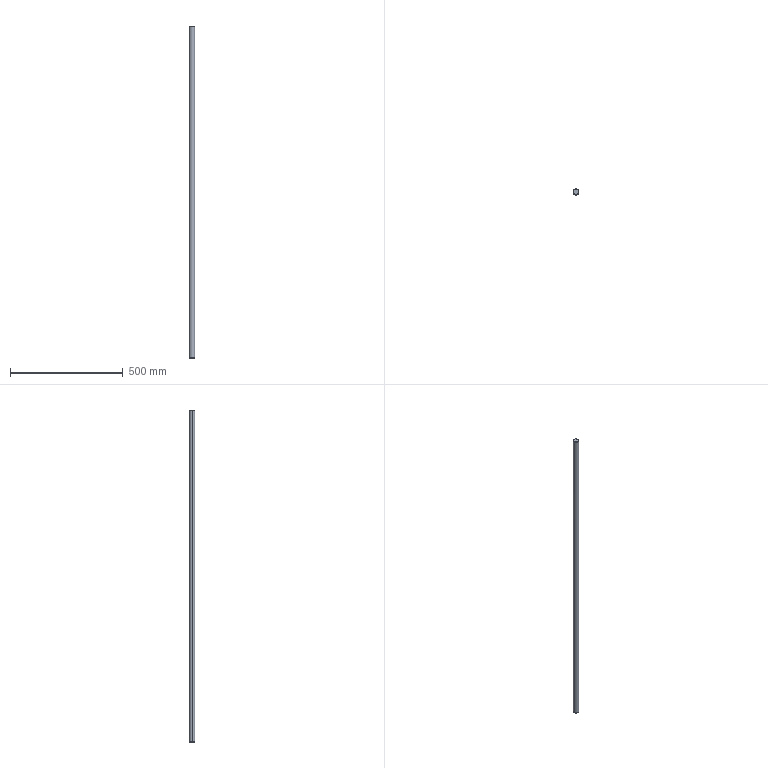Part | STEP file | 1 solid | 8 faces | box 25 x 25 x 1470 mm | volume 721508 mm3 | cone 4 | cylinder 2 | plane 2 | commonest cylinder face diameters 25 x2
STEP:
#1=CARTESIAN_POINT('',(0.,0.,0.));
#2=DIRECTION('',(0.,0.,1.));
#3=DIRECTION('',(1.,0.,0.));
#4=AXIS2_PLACEMENT_3D('',#1,#2,#3);
#5=CARTESIAN_POINT('',(-11.5,0.,-755.));
#6=VERTEX_POINT('',#5);
#7=CARTESIAN_POINT('',(11.5,0.,-755.));
#8=VERTEX_POINT('',#7);
#9=CARTESIAN_POINT('',(0.,0.,-755.));
#10=DIRECTION('',(0.,0.,-1.));
#11=DIRECTION('',(1.,0.,0.));
#12=AXIS2_PLACEMENT_3D('',#9,#10,#11);
#13=CIRCLE('',#12,11.5);
#14=CARTESIAN_POINT('',(0.,0.,-754.));
#15=DIRECTION('',(0.,0.,1.));
#16=DIRECTION('',(1.,0.,0.));
#17=AXIS2_PLACEMENT_3D('',#14,#15,#16);
#18=CONICAL_SURFACE('',#17,12.5,0.7854);
#19=CARTESIAN_POINT('',(6.283,-1.));
#20=DIRECTION('',(-1.,0.));
#21=VECTOR('',#20,1.);
#22=LINE('',#19,#21);
#23=(GEOMETRIC_REPRESENTATION_CONTEXT(2)PARAMETRIC_REPRESENTATION_CONTEXT()REPRESENTATION_CONTEXT('',''));
#24=DEFINITIONAL_REPRESENTATION('',(#22),#23);
#25=PCURVE('',#18,#24);
#26=CARTESIAN_POINT('',(0.,0.,-755.));
#27=DIRECTION('',(0.,0.,1.));
#28=DIRECTION('',(1.,0.,0.));
#29=AXIS2_PLACEMENT_3D('',#26,#27,#28);
#30=PLANE('',#29);
#31=CARTESIAN_POINT('',(11.5,0.));
#32=CARTESIAN_POINT('',(11.5,-19.919));
#33=CARTESIAN_POINT('',(-5.75,-9.959));
#34=CARTESIAN_POINT('',(-23.,0.));
#35=CARTESIAN_POINT('',(-5.75,9.959));
#36=CARTESIAN_POINT('',(11.5,19.919));
#37=CARTESIAN_POINT('',(11.5,0.));
#38=(BOUNDED_CURVE()B_SPLINE_CURVE(2,(#31,#32,#33,#34,#35,#36,#37),.UNSPECIFIED.,.T.,.F.)B_SPLINE_CURVE_WITH_KNOTS((1,2,2,2,2,1),(-2.094,0.,2.094,4.189,6.283,8.378),.UNSPECIFIED.)CURVE()GEOMETRIC_REPRESENTATION_ITEM()RATIONAL_B_SPLINE_CURVE((1.,0.5,1.,0.5,1.,0.5,1.))REPRESENTATION_ITEM(''));
#39=(GEOMETRIC_REPRESENTATION_CONTEXT(2)PARAMETRIC_REPRESENTATION_CONTEXT()REPRESENTATION_CONTEXT('',''));
#40=DEFINITIONAL_REPRESENTATION('',(#38),#39);
#41=PCURVE('',#30,#40);
#42=SURFACE_CURVE('',#13,(#25,#41),.PCURVE_S1.);
#43=EDGE_CURVE('',#6,#8,#42,.T.);
#44=ORIENTED_EDGE('',*,*,#43,.F.);
#45=CARTESIAN_POINT('',(-12.5,0.,-754.));
#46=VERTEX_POINT('',#45);
#47=CARTESIAN_POINT('',(-12.5,0.,-754.));
#48=DIRECTION('',(-0.7071,0.,0.7071));
#49=VECTOR('',#48,1.);
#50=LINE('',#47,#49);
#51=CARTESIAN_POINT('',(3.142,0.));
#52=DIRECTION('',(0.,1.));
#53=VECTOR('',#52,1.);
#54=LINE('',#51,#53);
#55=(GEOMETRIC_REPRESENTATION_CONTEXT(2)PARAMETRIC_REPRESENTATION_CONTEXT()REPRESENTATION_CONTEXT('',''));
#56=DEFINITIONAL_REPRESENTATION('',(#54),#55);
#57=PCURVE('',#18,#56);
#58=CARTESIAN_POINT('',(0.,0.,-754.));
#59=DIRECTION('',(0.,0.,1.));
#60=DIRECTION('',(1.,0.,0.));
#61=AXIS2_PLACEMENT_3D('',#58,#59,#60);
#62=CONICAL_SURFACE('',#61,12.5,0.7854);
#63=CARTESIAN_POINT('',(3.142,0.));
#64=DIRECTION('',(0.,1.));
#65=VECTOR('',#64,1.);
#66=LINE('',#63,#65);
#67=(GEOMETRIC_REPRESENTATION_CONTEXT(2)PARAMETRIC_REPRESENTATION_CONTEXT()REPRESENTATION_CONTEXT('',''));
#68=DEFINITIONAL_REPRESENTATION('',(#66),#67);
#69=PCURVE('',#62,#68);
#70=SURFACE_CURVE('',#50,(#57,#69),.PCURVE_S1.);
#71=EDGE_CURVE('',#6,#46,#70,.T.);
#72=ORIENTED_EDGE('',*,*,#71,.T.);
#73=CARTESIAN_POINT('',(12.5,0.,-754.));
#74=VERTEX_POINT('',#73);
#75=CARTESIAN_POINT('',(0.,0.,-754.));
#76=DIRECTION('',(0.,0.,1.));
#77=DIRECTION('',(1.,0.,0.));
#78=AXIS2_PLACEMENT_3D('',#75,#76,#77);
#79=CIRCLE('',#78,12.5);
#80=CARTESIAN_POINT('',(0.,0.));
#81=DIRECTION('',(1.,0.));
#82=VECTOR('',#81,1.);
#83=LINE('',#80,#82);
#84=(GEOMETRIC_REPRESENTATION_CONTEXT(2)PARAMETRIC_REPRESENTATION_CONTEXT()REPRESENTATION_CONTEXT('',''));
#85=DEFINITIONAL_REPRESENTATION('',(#83),#84);
#86=PCURVE('',#18,#85);
#87=CARTESIAN_POINT('',(0.,0.,755.));
#88=DIRECTION('',(0.,0.,-1.));
#89=DIRECTION('',(-1.,0.,0.));
#90=AXIS2_PLACEMENT_3D('',#87,#88,#89);
#91=CYLINDRICAL_SURFACE('',#90,12.5);
#92=CARTESIAN_POINT('',(3.142,1509.));
#93=DIRECTION('',(-1.,0.));
#94=VECTOR('',#93,1.);
#95=LINE('',#92,#94);
#96=(GEOMETRIC_REPRESENTATION_CONTEXT(2)PARAMETRIC_REPRESENTATION_CONTEXT()REPRESENTATION_CONTEXT('',''));
#97=DEFINITIONAL_REPRESENTATION('',(#95),#96);
#98=PCURVE('',#91,#97);
#99=SURFACE_CURVE('',#79,(#86,#98),.PCURVE_S1.);
#100=EDGE_CURVE('',#74,#46,#99,.T.);
#101=ORIENTED_EDGE('',*,*,#100,.F.);
#102=CARTESIAN_POINT('',(12.5,0.,-754.));
#103=DIRECTION('',(0.7071,0.,0.7071));
#104=VECTOR('',#103,1.);
#105=LINE('',#102,#104);
#106=CARTESIAN_POINT('',(0.,0.));
#107=DIRECTION('',(0.,1.));
#108=VECTOR('',#107,1.);
#109=LINE('',#106,#108);
#110=(GEOMETRIC_REPRESENTATION_CONTEXT(2)PARAMETRIC_REPRESENTATION_CONTEXT()REPRESENTATION_CONTEXT('',''));
#111=DEFINITIONAL_REPRESENTATION('',(#109),#110);
#112=PCURVE('',#18,#111);
#113=CARTESIAN_POINT('',(6.283,0.));
#114=DIRECTION('',(0.,1.));
#115=VECTOR('',#114,1.);
#116=LINE('',#113,#115);
#117=(GEOMETRIC_REPRESENTATION_CONTEXT(2)PARAMETRIC_REPRESENTATION_CONTEXT()REPRESENTATION_CONTEXT('',''));
#118=DEFINITIONAL_REPRESENTATION('',(#116),#117);
#119=PCURVE('',#62,#118);
#120=SURFACE_CURVE('',#105,(#112,#119),.PCURVE_S1.);
#121=EDGE_CURVE('',#8,#74,#120,.T.);
#122=ORIENTED_EDGE('',*,*,#121,.F.);
#123=EDGE_LOOP('',(#44,#72,#101,#122));
#124=FACE_BOUND('',#123,.T.);
#125=ADVANCED_FACE('',(#124),#18,.T.);
#126=CARTESIAN_POINT('',(11.5,0.,715.));
#127=VERTEX_POINT('',#126);
#128=CARTESIAN_POINT('',(-11.5,0.,715.));
#129=VERTEX_POINT('',#128);
#130=CARTESIAN_POINT('',(0.,0.,715.));
#131=DIRECTION('',(0.,0.,1.));
#132=DIRECTION('',(1.,0.,0.));
#133=AXIS2_PLACEMENT_3D('',#130,#131,#132);
#134=CIRCLE('',#133,11.5);
#135=CARTESIAN_POINT('',(0.,0.,715.));
#136=DIRECTION('',(0.,0.,-1.));
#137=DIRECTION('',(-1.,0.,0.));
#138=AXIS2_PLACEMENT_3D('',#135,#136,#137);
#139=CONICAL_SURFACE('',#138,11.5,0.7854);
#140=CARTESIAN_POINT('',(3.142,0.));
#141=DIRECTION('',(-1.,0.));
#142=VECTOR('',#141,1.);
#143=LINE('',#140,#142);
#144=(GEOMETRIC_REPRESENTATION_CONTEXT(2)PARAMETRIC_REPRESENTATION_CONTEXT()REPRESENTATION_CONTEXT('',''));
#145=DEFINITIONAL_REPRESENTATION('',(#143),#144);
#146=PCURVE('',#139,#145);
#147=CARTESIAN_POINT('',(0.,0.,715.));
#148=DIRECTION('',(0.,0.,1.));
#149=DIRECTION('',(1.,0.,0.));
#150=AXIS2_PLACEMENT_3D('',#147,#148,#149);
#151=PLANE('',#150);
#152=CARTESIAN_POINT('',(0.,0.));
#153=DIRECTION('',(1.,0.));
#154=AXIS2_PLACEMENT_2D('',#152,#153);
#155=CIRCLE('',#154,11.5);
#156=(GEOMETRIC_REPRESENTATION_CONTEXT(2)PARAMETRIC_REPRESENTATION_CONTEXT()REPRESENTATION_CONTEXT('',''));
#157=DEFINITIONAL_REPRESENTATION('',(#155),#156);
#158=PCURVE('',#151,#157);
#159=SURFACE_CURVE('',#134,(#146,#158),.PCURVE_S1.);
#160=EDGE_CURVE('',#127,#129,#159,.T.);
#161=ORIENTED_EDGE('',*,*,#160,.F.);
#162=CARTESIAN_POINT('',(12.5,0.,714.));
#163=VERTEX_POINT('',#162);
#164=CARTESIAN_POINT('',(11.5,0.,715.));
#165=DIRECTION('',(0.7071,0.,-0.7071));
#166=VECTOR('',#165,1.);
#167=LINE('',#164,#166);
#168=CARTESIAN_POINT('',(3.142,0.));
#169=DIRECTION('',(0.,1.));
#170=VECTOR('',#169,1.);
#171=LINE('',#168,#170);
#172=(GEOMETRIC_REPRESENTATION_CONTEXT(2)PARAMETRIC_REPRESENTATION_CONTEXT()REPRESENTATION_CONTEXT('',''));
#173=DEFINITIONAL_REPRESENTATION('',(#171),#172);
#174=PCURVE('',#139,#173);
#175=CARTESIAN_POINT('',(0.,0.,715.));
#176=DIRECTION('',(0.,0.,-1.));
#177=DIRECTION('',(-1.,0.,0.));
#178=AXIS2_PLACEMENT_3D('',#175,#176,#177);
#179=CONICAL_SURFACE('',#178,11.5,0.7854);
#180=CARTESIAN_POINT('',(3.142,0.));
#181=DIRECTION('',(0.,1.));
#182=VECTOR('',#181,1.);
#183=LINE('',#180,#182);
#184=(GEOMETRIC_REPRESENTATION_CONTEXT(2)PARAMETRIC_REPRESENTATION_CONTEXT()REPRESENTATION_CONTEXT('',''));
#185=DEFINITIONAL_REPRESENTATION('',(#183),#184);
#186=PCURVE('',#179,#185);
#187=SURFACE_CURVE('',#167,(#174,#186),.PCURVE_S1.);
#188=EDGE_CURVE('',#127,#163,#187,.T.);
#189=ORIENTED_EDGE('',*,*,#188,.T.);
#190=CARTESIAN_POINT('',(-12.5,0.,714.));
#191=VERTEX_POINT('',#190);
#192=CARTESIAN_POINT('',(0.,0.,714.));
#193=DIRECTION('',(0.,0.,-1.));
#194=DIRECTION('',(1.,0.,0.));
#195=AXIS2_PLACEMENT_3D('',#192,#193,#194);
#196=CIRCLE('',#195,12.5);
#197=CARTESIAN_POINT('',(-3.142,1.));
#198=DIRECTION('',(1.,0.));
#199=VECTOR('',#198,1.);
#200=LINE('',#197,#199);
#201=(GEOMETRIC_REPRESENTATION_CONTEXT(2)PARAMETRIC_REPRESENTATION_CONTEXT()REPRESENTATION_CONTEXT('',''));
#202=DEFINITIONAL_REPRESENTATION('',(#200),#201);
#203=PCURVE('',#139,#202);
#204=CARTESIAN_POINT('',(-3.142,41.));
#205=DIRECTION('',(1.,0.));
#206=VECTOR('',#205,1.);
#207=LINE('',#204,#206);
#208=(GEOMETRIC_REPRESENTATION_CONTEXT(2)PARAMETRIC_REPRESENTATION_CONTEXT()REPRESENTATION_CONTEXT('',''));
#209=DEFINITIONAL_REPRESENTATION('',(#207),#208);
#210=PCURVE('',#91,#209);
#211=SURFACE_CURVE('',#196,(#203,#210),.PCURVE_S1.);
#212=EDGE_CURVE('',#191,#163,#211,.T.);
#213=ORIENTED_EDGE('',*,*,#212,.F.);
#214=CARTESIAN_POINT('',(-11.5,0.,715.));
#215=DIRECTION('',(-0.7071,0.,-0.7071));
#216=VECTOR('',#215,1.);
#217=LINE('',#214,#216);
#218=CARTESIAN_POINT('',(0.,0.));
#219=DIRECTION('',(0.,1.));
#220=VECTOR('',#219,1.);
#221=LINE('',#218,#220);
#222=(GEOMETRIC_REPRESENTATION_CONTEXT(2)PARAMETRIC_REPRESENTATION_CONTEXT()REPRESENTATION_CONTEXT('',''));
#223=DEFINITIONAL_REPRESENTATION('',(#221),#222);
#224=PCURVE('',#139,#223);
#225=CARTESIAN_POINT('',(6.283,0.));
#226=DIRECTION('',(0.,1.));
#227=VECTOR('',#226,1.);
#228=LINE('',#225,#227);
#229=(GEOMETRIC_REPRESENTATION_CONTEXT(2)PARAMETRIC_REPRESENTATION_CONTEXT()REPRESENTATION_CONTEXT('',''));
#230=DEFINITIONAL_REPRESENTATION('',(#228),#229);
#231=PCURVE('',#179,#230);
#232=SURFACE_CURVE('',#217,(#224,#231),.PCURVE_S1.);
#233=EDGE_CURVE('',#129,#191,#232,.T.);
#234=ORIENTED_EDGE('',*,*,#233,.F.);
#235=EDGE_LOOP('',(#161,#189,#213,#234));
#236=FACE_BOUND('',#235,.T.);
#237=ADVANCED_FACE('',(#236),#139,.T.);
#238=ORIENTED_EDGE('',*,*,#212,.T.);
#239=CARTESIAN_POINT('',(12.5,0.,755.));
#240=DIRECTION('',(0.,0.,-1.));
#241=VECTOR('',#240,1.);
#242=LINE('',#239,#241);
#243=CARTESIAN_POINT('',(3.142,0.));
#244=DIRECTION('',(0.,1.));
#245=VECTOR('',#244,1.);
#246=LINE('',#243,#245);
#247=(GEOMETRIC_REPRESENTATION_CONTEXT(2)PARAMETRIC_REPRESENTATION_CONTEXT()REPRESENTATION_CONTEXT('',''));
#248=DEFINITIONAL_REPRESENTATION('',(#246),#247);
#249=PCURVE('',#91,#248);
#250=CARTESIAN_POINT('',(0.,0.,755.));
#251=DIRECTION('',(0.,0.,-1.));
#252=DIRECTION('',(-1.,0.,0.));
#253=AXIS2_PLACEMENT_3D('',#250,#251,#252);
#254=CYLINDRICAL_SURFACE('',#253,12.5);
#255=CARTESIAN_POINT('',(3.142,0.));
#256=DIRECTION('',(0.,1.));
#257=VECTOR('',#256,1.);
#258=LINE('',#255,#257);
#259=(GEOMETRIC_REPRESENTATION_CONTEXT(2)PARAMETRIC_REPRESENTATION_CONTEXT()REPRESENTATION_CONTEXT('',''));
#260=DEFINITIONAL_REPRESENTATION('',(#258),#259);
#261=PCURVE('',#254,#260);
#262=SURFACE_CURVE('',#242,(#249,#261),.PCURVE_S1.);
#263=EDGE_CURVE('',#163,#74,#262,.T.);
#264=ORIENTED_EDGE('',*,*,#263,.T.);
#265=ORIENTED_EDGE('',*,*,#100,.T.);
#266=CARTESIAN_POINT('',(-12.5,0.,755.));
#267=DIRECTION('',(0.,0.,-1.));
#268=VECTOR('',#267,1.);
#269=LINE('',#266,#268);
#270=CARTESIAN_POINT('',(0.,0.));
#271=DIRECTION('',(0.,1.));
#272=VECTOR('',#271,1.);
#273=LINE('',#270,#272);
#274=(GEOMETRIC_REPRESENTATION_CONTEXT(2)PARAMETRIC_REPRESENTATION_CONTEXT()REPRESENTATION_CONTEXT('',''));
#275=DEFINITIONAL_REPRESENTATION('',(#273),#274);
#276=PCURVE('',#91,#275);
#277=CARTESIAN_POINT('',(6.283,0.));
#278=DIRECTION('',(0.,1.));
#279=VECTOR('',#278,1.);
#280=LINE('',#277,#279);
#281=(GEOMETRIC_REPRESENTATION_CONTEXT(2)PARAMETRIC_REPRESENTATION_CONTEXT()REPRESENTATION_CONTEXT('',''));
#282=DEFINITIONAL_REPRESENTATION('',(#280),#281);
#283=PCURVE('',#254,#282);
#284=SURFACE_CURVE('',#269,(#276,#283),.PCURVE_S1.);
#285=EDGE_CURVE('',#191,#46,#284,.T.);
#286=ORIENTED_EDGE('',*,*,#285,.F.);
#287=EDGE_LOOP('',(#238,#264,#265,#286));
#288=FACE_BOUND('',#287,.T.);
#289=ADVANCED_FACE('',(#288),#91,.T.);
#290=ORIENTED_EDGE('',*,*,#263,.F.);
#291=CARTESIAN_POINT('',(0.,0.,714.));
#292=DIRECTION('',(0.,0.,-1.));
#293=DIRECTION('',(1.,0.,0.));
#294=AXIS2_PLACEMENT_3D('',#291,#292,#293);
#295=CIRCLE('',#294,12.5);
#296=CARTESIAN_POINT('',(3.142,41.));
#297=DIRECTION('',(1.,0.));
#298=VECTOR('',#297,1.);
#299=LINE('',#296,#298);
#300=(GEOMETRIC_REPRESENTATION_CONTEXT(2)PARAMETRIC_REPRESENTATION_CONTEXT()REPRESENTATION_CONTEXT('',''));
#301=DEFINITIONAL_REPRESENTATION('',(#299),#300);
#302=PCURVE('',#254,#301);
#303=CARTESIAN_POINT('',(3.142,1.));
#304=DIRECTION('',(1.,0.));
#305=VECTOR('',#304,1.);
#306=LINE('',#303,#305);
#307=(GEOMETRIC_REPRESENTATION_CONTEXT(2)PARAMETRIC_REPRESENTATION_CONTEXT()REPRESENTATION_CONTEXT('',''));
#308=DEFINITIONAL_REPRESENTATION('',(#306),#307);
#309=PCURVE('',#179,#308);
#310=SURFACE_CURVE('',#295,(#302,#309),.PCURVE_S1.);
#311=EDGE_CURVE('',#163,#191,#310,.T.);
#312=ORIENTED_EDGE('',*,*,#311,.T.);
#313=ORIENTED_EDGE('',*,*,#285,.T.);
#314=CARTESIAN_POINT('',(0.,0.,-754.));
#315=DIRECTION('',(0.,0.,1.));
#316=DIRECTION('',(1.,0.,0.));
#317=AXIS2_PLACEMENT_3D('',#314,#315,#316);
#318=CIRCLE('',#317,12.5);
#319=CARTESIAN_POINT('',(9.425,1509.));
#320=DIRECTION('',(-1.,0.));
#321=VECTOR('',#320,1.);
#322=LINE('',#319,#321);
#323=(GEOMETRIC_REPRESENTATION_CONTEXT(2)PARAMETRIC_REPRESENTATION_CONTEXT()REPRESENTATION_CONTEXT('',''));
#324=DEFINITIONAL_REPRESENTATION('',(#322),#323);
#325=PCURVE('',#254,#324);
#326=CARTESIAN_POINT('',(0.,0.));
#327=DIRECTION('',(1.,0.));
#328=VECTOR('',#327,1.);
#329=LINE('',#326,#328);
#330=(GEOMETRIC_REPRESENTATION_CONTEXT(2)PARAMETRIC_REPRESENTATION_CONTEXT()REPRESENTATION_CONTEXT('',''));
#331=DEFINITIONAL_REPRESENTATION('',(#329),#330);
#332=PCURVE('',#62,#331);
#333=SURFACE_CURVE('',#318,(#325,#332),.PCURVE_S1.);
#334=EDGE_CURVE('',#46,#74,#333,.T.);
#335=ORIENTED_EDGE('',*,*,#334,.T.);
#336=EDGE_LOOP('',(#290,#312,#313,#335));
#337=FACE_BOUND('',#336,.T.);
#338=ADVANCED_FACE('',(#337),#254,.T.);
#339=CARTESIAN_POINT('',(0.,0.,715.));
#340=DIRECTION('',(0.,0.,1.));
#341=DIRECTION('',(1.,0.,0.));
#342=AXIS2_PLACEMENT_3D('',#339,#340,#341);
#343=CIRCLE('',#342,11.5);
#344=CARTESIAN_POINT('',(0.,0.));
#345=DIRECTION('',(1.,0.));
#346=AXIS2_PLACEMENT_2D('',#344,#345);
#347=CIRCLE('',#346,11.5);
#348=(GEOMETRIC_REPRESENTATION_CONTEXT(2)PARAMETRIC_REPRESENTATION_CONTEXT()REPRESENTATION_CONTEXT('',''));
#349=DEFINITIONAL_REPRESENTATION('',(#347),#348);
#350=PCURVE('',#151,#349);
#351=CARTESIAN_POINT('',(9.425,0.));
#352=DIRECTION('',(-1.,0.));
#353=VECTOR('',#352,1.);
#354=LINE('',#351,#353);
#355=(GEOMETRIC_REPRESENTATION_CONTEXT(2)PARAMETRIC_REPRESENTATION_CONTEXT()REPRESENTATION_CONTEXT('',''));
#356=DEFINITIONAL_REPRESENTATION('',(#354),#355);
#357=PCURVE('',#179,#356);
#358=SURFACE_CURVE('',#343,(#350,#357),.PCURVE_S1.);
#359=EDGE_CURVE('',#129,#127,#358,.T.);
#360=ORIENTED_EDGE('',*,*,#359,.T.);
#361=ORIENTED_EDGE('',*,*,#160,.T.);
#362=EDGE_LOOP('',(#360,#361));
#363=FACE_BOUND('',#362,.T.);
#364=ADVANCED_FACE('',(#363),#151,.T.);
#365=CARTESIAN_POINT('',(0.,0.,-755.));
#366=DIRECTION('',(0.,0.,-1.));
#367=DIRECTION('',(1.,0.,0.));
#368=AXIS2_PLACEMENT_3D('',#365,#366,#367);
#369=CIRCLE('',#368,11.5);
#370=CARTESIAN_POINT('',(11.5,0.));
#371=CARTESIAN_POINT('',(11.5,-19.919));
#372=CARTESIAN_POINT('',(-5.75,-9.959));
#373=CARTESIAN_POINT('',(-23.,0.));
#374=CARTESIAN_POINT('',(-5.75,9.959));
#375=CARTESIAN_POINT('',(11.5,19.919));
#376=CARTESIAN_POINT('',(11.5,0.));
#377=(BOUNDED_CURVE()B_SPLINE_CURVE(2,(#370,#371,#372,#373,#374,#375,#376),.UNSPECIFIED.,.T.,.F.)B_SPLINE_CURVE_WITH_KNOTS((1,2,2,2,2,1),(-2.094,0.,2.094,4.189,6.283,8.378),.UNSPECIFIED.)CURVE()GEOMETRIC_REPRESENTATION_ITEM()RATIONAL_B_SPLINE_CURVE((1.,0.5,1.,0.5,1.,0.5,1.))REPRESENTATION_ITEM(''));
#378=(GEOMETRIC_REPRESENTATION_CONTEXT(2)PARAMETRIC_REPRESENTATION_CONTEXT()REPRESENTATION_CONTEXT('',''));
#379=DEFINITIONAL_REPRESENTATION('',(#377),#378);
#380=PCURVE('',#30,#379);
#381=CARTESIAN_POINT('',(6.283,-1.));
#382=DIRECTION('',(-1.,0.));
#383=VECTOR('',#382,1.);
#384=LINE('',#381,#383);
#385=(GEOMETRIC_REPRESENTATION_CONTEXT(2)PARAMETRIC_REPRESENTATION_CONTEXT()REPRESENTATION_CONTEXT('',''));
#386=DEFINITIONAL_REPRESENTATION('',(#384),#385);
#387=PCURVE('',#62,#386);
#388=SURFACE_CURVE('',#369,(#380,#387),.PCURVE_S1.);
#389=EDGE_CURVE('',#8,#6,#388,.T.);
#390=ORIENTED_EDGE('',*,*,#389,.T.);
#391=ORIENTED_EDGE('',*,*,#43,.T.);
#392=EDGE_LOOP('',(#390,#391));
#393=FACE_BOUND('',#392,.T.);
#394=ADVANCED_FACE('',(#393),#30,.F.);
#395=ORIENTED_EDGE('',*,*,#188,.F.);
#396=ORIENTED_EDGE('',*,*,#359,.F.);
#397=ORIENTED_EDGE('',*,*,#233,.T.);
#398=ORIENTED_EDGE('',*,*,#311,.F.);
#399=EDGE_LOOP('',(#395,#396,#397,#398));
#400=FACE_BOUND('',#399,.T.);
#401=ADVANCED_FACE('',(#400),#179,.T.);
#402=ORIENTED_EDGE('',*,*,#71,.F.);
#403=ORIENTED_EDGE('',*,*,#389,.F.);
#404=ORIENTED_EDGE('',*,*,#121,.T.);
#405=ORIENTED_EDGE('',*,*,#334,.F.);
#406=EDGE_LOOP('',(#402,#403,#404,#405));
#407=FACE_BOUND('',#406,.T.);
#408=ADVANCED_FACE('',(#407),#62,.T.);
#409=CLOSED_SHELL('',(#125,#237,#289,#338,#364,#394,#401,#408));
#410=MANIFOLD_SOLID_BREP('',#409);
#411=(LENGTH_UNIT()NAMED_UNIT(*)SI_UNIT(.MILLI.,.METRE.));
#412=UNCERTAINTY_MEASURE_WITH_UNIT(LENGTH_MEASURE(0.0000001),#411,'','');
#413=(NAMED_UNIT(*)PLANE_ANGLE_UNIT()SI_UNIT($,.RADIAN.));
#414=(NAMED_UNIT(*)SI_UNIT($,.STERADIAN.)SOLID_ANGLE_UNIT());
#415=(GEOMETRIC_REPRESENTATION_CONTEXT(3)GLOBAL_UNCERTAINTY_ASSIGNED_CONTEXT((#412))GLOBAL_UNIT_ASSIGNED_CONTEXT((#411,#413,#414))REPRESENTATION_CONTEXT('',''));
#416=ADVANCED_BREP_SHAPE_REPRESENTATION('',(#4,#410),#415);